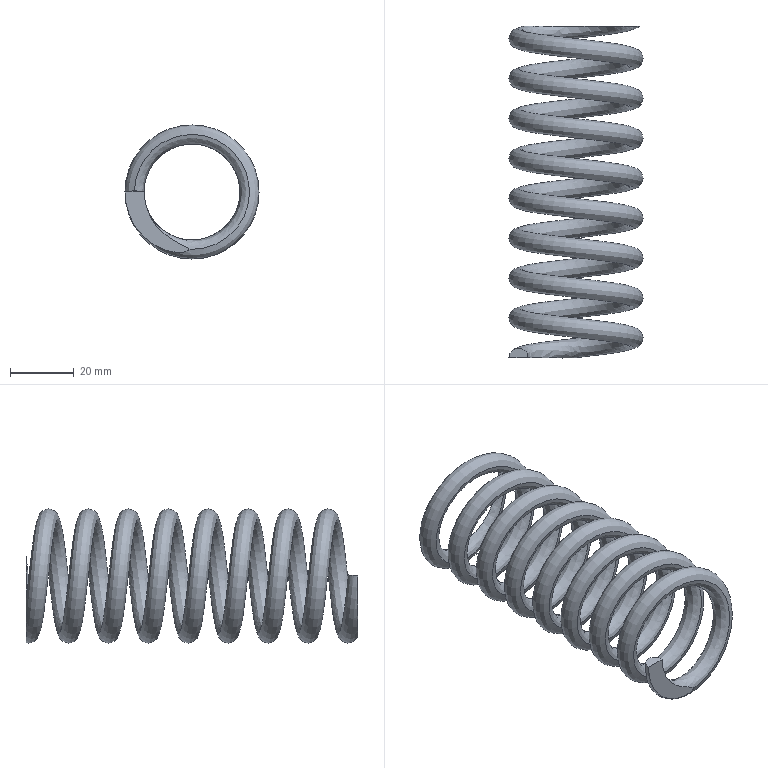Part | SolidWorks | features Helix 1, ICE 1, Sweep 1 | 1 solid | 5 faces | box 42 x 103.92 x 42 mm | volume 26599 mm3 | plane 3 | spline 2